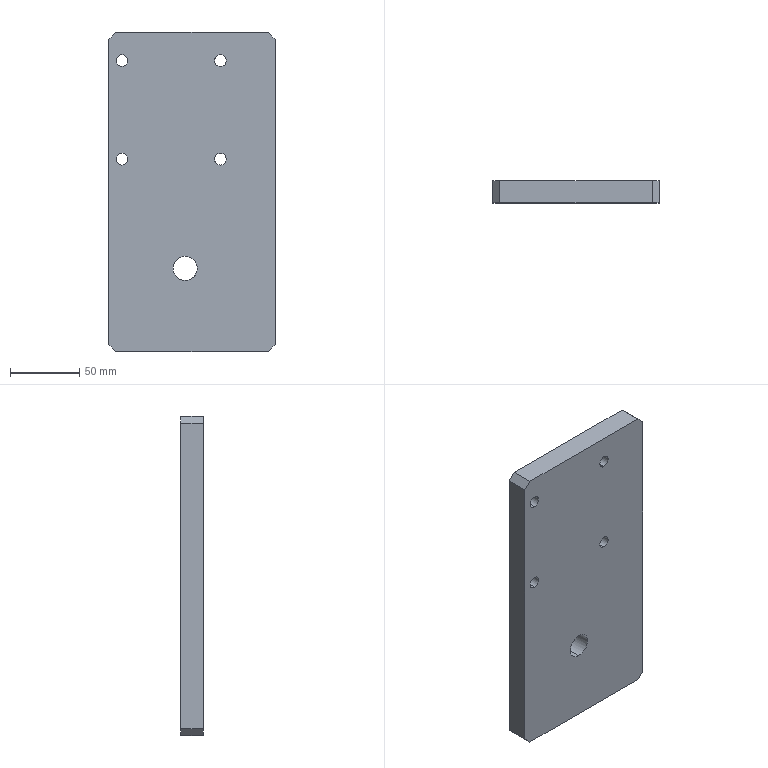Part | STEP file | 1 solid | 30 faces | box 120 x 16 x 230 mm | volume 433239 mm3 | cone 10 | cylinder 10 | plane 10 | commonest cylinder face diameters 8.5 x8 17.5 x2